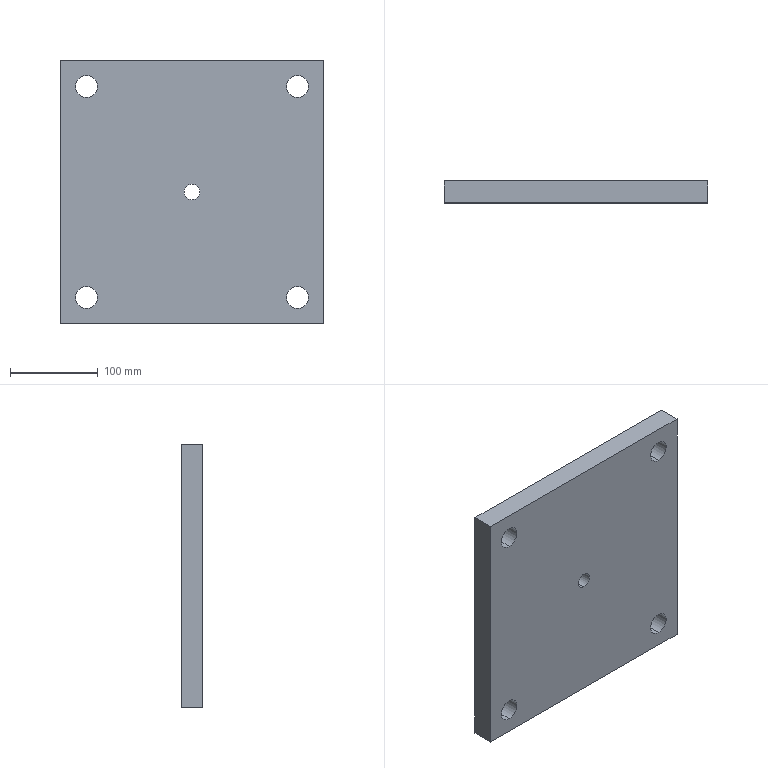Part | SolidWorks | features FlatPattern 1, SMBaseFlange 1, SheetMetal 1 | 1 solid | 16 faces | box 300 x 25 x 300 mm | volume 2194551 mm3 | cylinder 10 | plane 6 | commonest cylinder face diameters 25 x8 18 x2
STEP:
#1=CARTESIAN_POINT('',(-120.,-25.,-132.5));
#2=VERTEX_POINT('',#1);
#3=CARTESIAN_POINT('',(-120.,-25.,-107.5));
#4=VERTEX_POINT('',#3);
#5=CARTESIAN_POINT('',(-120.,-25.,-120.));
#6=DIRECTION('',(0.,1.,0.));
#7=DIRECTION('',(0.,0.,-1.));
#8=AXIS2_PLACEMENT_3D('',#5,#6,#7);
#9=CIRCLE('',#8,12.5);
#10=EDGE_CURVE('',#2,#4,#9,.T.);
#11=ORIENTED_EDGE('',*,*,#10,.F.);
#12=CARTESIAN_POINT('',(-120.,0.,-132.5));
#13=VERTEX_POINT('',#12);
#14=CARTESIAN_POINT('',(-120.,-25.,-132.5));
#15=DIRECTION('',(0.,1.,0.));
#16=VECTOR('',#15,1000.);
#17=LINE('',#14,#16);
#18=EDGE_CURVE('',#2,#13,#17,.T.);
#19=ORIENTED_EDGE('',*,*,#18,.T.);
#20=CARTESIAN_POINT('',(-120.,0.,-107.5));
#21=VERTEX_POINT('',#20);
#22=CARTESIAN_POINT('',(-120.,0.,-120.));
#23=DIRECTION('',(0.,1.,0.));
#24=DIRECTION('',(0.,0.,-1.));
#25=AXIS2_PLACEMENT_3D('',#22,#23,#24);
#26=CIRCLE('',#25,12.5);
#27=EDGE_CURVE('',#13,#21,#26,.T.);
#28=ORIENTED_EDGE('',*,*,#27,.T.);
#29=CARTESIAN_POINT('',(-120.,-25.,-107.5));
#30=DIRECTION('',(0.,1.,0.));
#31=VECTOR('',#30,1000.);
#32=LINE('',#29,#31);
#33=EDGE_CURVE('',#4,#21,#32,.T.);
#34=ORIENTED_EDGE('',*,*,#33,.F.);
#35=EDGE_LOOP('',(#11,#19,#28,#34));
#36=FACE_OUTER_BOUND('',#35,.T.);
#37=CARTESIAN_POINT('',(-120.,-25.,-120.));
#38=DIRECTION('',(0.,1.,0.));
#39=DIRECTION('',(0.,0.,1.));
#40=AXIS2_PLACEMENT_3D('',#37,#38,#39);
#41=CYLINDRICAL_SURFACE('',#40,12.5);
#42=ADVANCED_FACE('',(#36),#41,.F.);
#43=CARTESIAN_POINT('',(120.,-25.,-132.5));
#44=VERTEX_POINT('',#43);
#45=CARTESIAN_POINT('',(120.,-25.,-107.5));
#46=VERTEX_POINT('',#45);
#47=CARTESIAN_POINT('',(120.,-25.,-120.));
#48=DIRECTION('',(0.,1.,0.));
#49=DIRECTION('',(0.,0.,1.));
#50=AXIS2_PLACEMENT_3D('',#47,#48,#49);
#51=CIRCLE('',#50,12.5);
#52=EDGE_CURVE('',#44,#46,#51,.T.);
#53=ORIENTED_EDGE('',*,*,#52,.F.);
#54=CARTESIAN_POINT('',(120.,0.,-132.5));
#55=VERTEX_POINT('',#54);
#56=CARTESIAN_POINT('',(120.,-25.,-132.5));
#57=DIRECTION('',(0.,1.,0.));
#58=VECTOR('',#57,1000.);
#59=LINE('',#56,#58);
#60=EDGE_CURVE('',#44,#55,#59,.T.);
#61=ORIENTED_EDGE('',*,*,#60,.T.);
#62=CARTESIAN_POINT('',(120.,0.,-107.5));
#63=VERTEX_POINT('',#62);
#64=CARTESIAN_POINT('',(120.,0.,-120.));
#65=DIRECTION('',(0.,1.,0.));
#66=DIRECTION('',(0.,0.,1.));
#67=AXIS2_PLACEMENT_3D('',#64,#65,#66);
#68=CIRCLE('',#67,12.5);
#69=EDGE_CURVE('',#55,#63,#68,.T.);
#70=ORIENTED_EDGE('',*,*,#69,.T.);
#71=CARTESIAN_POINT('',(120.,-25.,-107.5));
#72=DIRECTION('',(0.,1.,0.));
#73=VECTOR('',#72,1000.);
#74=LINE('',#71,#73);
#75=EDGE_CURVE('',#46,#63,#74,.T.);
#76=ORIENTED_EDGE('',*,*,#75,.F.);
#77=EDGE_LOOP('',(#53,#61,#70,#76));
#78=FACE_OUTER_BOUND('',#77,.T.);
#79=CARTESIAN_POINT('',(120.,-25.,-120.));
#80=DIRECTION('',(0.,1.,0.));
#81=DIRECTION('',(0.,0.,1.));
#82=AXIS2_PLACEMENT_3D('',#79,#80,#81);
#83=CYLINDRICAL_SURFACE('',#82,12.5);
#84=ADVANCED_FACE('',(#78),#83,.F.);
#85=CARTESIAN_POINT('',(0.,-25.,-9.));
#86=VERTEX_POINT('',#85);
#87=CARTESIAN_POINT('',(0.,-25.,9.));
#88=VERTEX_POINT('',#87);
#89=CARTESIAN_POINT('',(0.,-25.,0.));
#90=DIRECTION('',(0.,1.,0.));
#91=DIRECTION('',(0.,0.,1.));
#92=AXIS2_PLACEMENT_3D('',#89,#90,#91);
#93=CIRCLE('',#92,9.);
#94=EDGE_CURVE('',#86,#88,#93,.T.);
#95=ORIENTED_EDGE('',*,*,#94,.F.);
#96=CARTESIAN_POINT('',(0.,0.,-9.));
#97=VERTEX_POINT('',#96);
#98=CARTESIAN_POINT('',(0.,-25.,-9.));
#99=DIRECTION('',(0.,1.,0.));
#100=VECTOR('',#99,1000.);
#101=LINE('',#98,#100);
#102=EDGE_CURVE('',#86,#97,#101,.T.);
#103=ORIENTED_EDGE('',*,*,#102,.T.);
#104=CARTESIAN_POINT('',(0.,0.,9.));
#105=VERTEX_POINT('',#104);
#106=CARTESIAN_POINT('',(0.,0.,0.));
#107=DIRECTION('',(0.,1.,0.));
#108=DIRECTION('',(0.,0.,1.));
#109=AXIS2_PLACEMENT_3D('',#106,#107,#108);
#110=CIRCLE('',#109,9.);
#111=EDGE_CURVE('',#97,#105,#110,.T.);
#112=ORIENTED_EDGE('',*,*,#111,.T.);
#113=CARTESIAN_POINT('',(0.,-25.,9.));
#114=DIRECTION('',(0.,1.,0.));
#115=VECTOR('',#114,1000.);
#116=LINE('',#113,#115);
#117=EDGE_CURVE('',#88,#105,#116,.T.);
#118=ORIENTED_EDGE('',*,*,#117,.F.);
#119=EDGE_LOOP('',(#95,#103,#112,#118));
#120=FACE_OUTER_BOUND('',#119,.T.);
#121=CARTESIAN_POINT('',(0.,-25.,0.));
#122=DIRECTION('',(0.,1.,0.));
#123=DIRECTION('',(0.,0.,1.));
#124=AXIS2_PLACEMENT_3D('',#121,#122,#123);
#125=CYLINDRICAL_SURFACE('',#124,9.);
#126=ADVANCED_FACE('',(#120),#125,.F.);
#127=CARTESIAN_POINT('',(120.,-25.,107.5));
#128=VERTEX_POINT('',#127);
#129=CARTESIAN_POINT('',(120.,-25.,132.5));
#130=VERTEX_POINT('',#129);
#131=CARTESIAN_POINT('',(120.,-25.,120.));
#132=DIRECTION('',(0.,1.,0.));
#133=DIRECTION('',(0.,0.,-1.));
#134=AXIS2_PLACEMENT_3D('',#131,#132,#133);
#135=CIRCLE('',#134,12.5);
#136=EDGE_CURVE('',#128,#130,#135,.T.);
#137=ORIENTED_EDGE('',*,*,#136,.F.);
#138=CARTESIAN_POINT('',(120.,0.,107.5));
#139=VERTEX_POINT('',#138);
#140=CARTESIAN_POINT('',(120.,-25.,107.5));
#141=DIRECTION('',(0.,1.,0.));
#142=VECTOR('',#141,1000.);
#143=LINE('',#140,#142);
#144=EDGE_CURVE('',#128,#139,#143,.T.);
#145=ORIENTED_EDGE('',*,*,#144,.T.);
#146=CARTESIAN_POINT('',(120.,0.,132.5));
#147=VERTEX_POINT('',#146);
#148=CARTESIAN_POINT('',(120.,0.,120.));
#149=DIRECTION('',(0.,1.,0.));
#150=DIRECTION('',(0.,0.,-1.));
#151=AXIS2_PLACEMENT_3D('',#148,#149,#150);
#152=CIRCLE('',#151,12.5);
#153=EDGE_CURVE('',#139,#147,#152,.T.);
#154=ORIENTED_EDGE('',*,*,#153,.T.);
#155=CARTESIAN_POINT('',(120.,-25.,132.5));
#156=DIRECTION('',(0.,1.,0.));
#157=VECTOR('',#156,1000.);
#158=LINE('',#155,#157);
#159=EDGE_CURVE('',#130,#147,#158,.T.);
#160=ORIENTED_EDGE('',*,*,#159,.F.);
#161=EDGE_LOOP('',(#137,#145,#154,#160));
#162=FACE_OUTER_BOUND('',#161,.T.);
#163=CARTESIAN_POINT('',(120.,-25.,120.));
#164=DIRECTION('',(0.,1.,0.));
#165=DIRECTION('',(0.,0.,1.));
#166=AXIS2_PLACEMENT_3D('',#163,#164,#165);
#167=CYLINDRICAL_SURFACE('',#166,12.5);
#168=ADVANCED_FACE('',(#162),#167,.F.);
#169=CARTESIAN_POINT('',(-120.,-25.,107.5));
#170=VERTEX_POINT('',#169);
#171=CARTESIAN_POINT('',(-120.,-25.,132.5));
#172=VERTEX_POINT('',#171);
#173=CARTESIAN_POINT('',(-120.,-25.,120.));
#174=DIRECTION('',(0.,1.,0.));
#175=DIRECTION('',(0.,0.,1.));
#176=AXIS2_PLACEMENT_3D('',#173,#174,#175);
#177=CIRCLE('',#176,12.5);
#178=EDGE_CURVE('',#170,#172,#177,.T.);
#179=ORIENTED_EDGE('',*,*,#178,.F.);
#180=CARTESIAN_POINT('',(-120.,0.,107.5));
#181=VERTEX_POINT('',#180);
#182=CARTESIAN_POINT('',(-120.,-25.,107.5));
#183=DIRECTION('',(0.,1.,0.));
#184=VECTOR('',#183,1000.);
#185=LINE('',#182,#184);
#186=EDGE_CURVE('',#170,#181,#185,.T.);
#187=ORIENTED_EDGE('',*,*,#186,.T.);
#188=CARTESIAN_POINT('',(-120.,0.,132.5));
#189=VERTEX_POINT('',#188);
#190=CARTESIAN_POINT('',(-120.,0.,120.));
#191=DIRECTION('',(0.,1.,0.));
#192=DIRECTION('',(0.,0.,1.));
#193=AXIS2_PLACEMENT_3D('',#190,#191,#192);
#194=CIRCLE('',#193,12.5);
#195=EDGE_CURVE('',#181,#189,#194,.T.);
#196=ORIENTED_EDGE('',*,*,#195,.T.);
#197=CARTESIAN_POINT('',(-120.,-25.,132.5));
#198=DIRECTION('',(0.,1.,0.));
#199=VECTOR('',#198,1000.);
#200=LINE('',#197,#199);
#201=EDGE_CURVE('',#172,#189,#200,.T.);
#202=ORIENTED_EDGE('',*,*,#201,.F.);
#203=EDGE_LOOP('',(#179,#187,#196,#202));
#204=FACE_OUTER_BOUND('',#203,.T.);
#205=CARTESIAN_POINT('',(-120.,-25.,120.));
#206=DIRECTION('',(0.,1.,0.));
#207=DIRECTION('',(0.,0.,1.));
#208=AXIS2_PLACEMENT_3D('',#205,#206,#207);
#209=CYLINDRICAL_SURFACE('',#208,12.5);
#210=ADVANCED_FACE('',(#204),#209,.F.);
#211=CARTESIAN_POINT('',(150.,0.,150.));
#212=VERTEX_POINT('',#211);
#213=CARTESIAN_POINT('',(150.,0.,-150.));
#214=VERTEX_POINT('',#213);
#215=CARTESIAN_POINT('',(150.,0.,-150.));
#216=DIRECTION('',(0.,0.,-1.));
#217=VECTOR('',#216,1000.);
#218=LINE('',#215,#217);
#219=EDGE_CURVE('',#212,#214,#218,.T.);
#220=ORIENTED_EDGE('',*,*,#219,.F.);
#221=CARTESIAN_POINT('',(150.,-25.,150.));
#222=VERTEX_POINT('',#221);
#223=CARTESIAN_POINT('',(150.,-25.,150.));
#224=DIRECTION('',(0.,1.,0.));
#225=VECTOR('',#224,1000.);
#226=LINE('',#223,#225);
#227=EDGE_CURVE('',#222,#212,#226,.T.);
#228=ORIENTED_EDGE('',*,*,#227,.F.);
#229=CARTESIAN_POINT('',(150.,-25.,-150.));
#230=VERTEX_POINT('',#229);
#231=CARTESIAN_POINT('',(150.,-25.,-150.));
#232=DIRECTION('',(0.,0.,-1.));
#233=VECTOR('',#232,1000.);
#234=LINE('',#231,#233);
#235=EDGE_CURVE('',#222,#230,#234,.T.);
#236=ORIENTED_EDGE('',*,*,#235,.T.);
#237=CARTESIAN_POINT('',(150.,-25.,-150.));
#238=DIRECTION('',(0.,1.,0.));
#239=VECTOR('',#238,1000.);
#240=LINE('',#237,#239);
#241=EDGE_CURVE('',#230,#214,#240,.T.);
#242=ORIENTED_EDGE('',*,*,#241,.T.);
#243=EDGE_LOOP('',(#220,#228,#236,#242));
#244=FACE_OUTER_BOUND('',#243,.T.);
#245=CARTESIAN_POINT('',(150.,-25.,-150.));
#246=DIRECTION('',(1.,0.,0.));
#247=DIRECTION('',(0.,0.,-1.));
#248=AXIS2_PLACEMENT_3D('',#245,#246,#247);
#249=PLANE('',#248);
#250=ADVANCED_FACE('',(#244),#249,.T.);
#251=CARTESIAN_POINT('',(-150.,0.,150.));
#252=VERTEX_POINT('',#251);
#253=CARTESIAN_POINT('',(-150.,0.,150.));
#254=DIRECTION('',(1.,0.,0.));
#255=VECTOR('',#254,1000.);
#256=LINE('',#253,#255);
#257=EDGE_CURVE('',#252,#212,#256,.T.);
#258=ORIENTED_EDGE('',*,*,#257,.F.);
#259=CARTESIAN_POINT('',(-150.,-25.,150.));
#260=VERTEX_POINT('',#259);
#261=CARTESIAN_POINT('',(-150.,-25.,150.));
#262=DIRECTION('',(0.,1.,0.));
#263=VECTOR('',#262,1000.);
#264=LINE('',#261,#263);
#265=EDGE_CURVE('',#260,#252,#264,.T.);
#266=ORIENTED_EDGE('',*,*,#265,.F.);
#267=CARTESIAN_POINT('',(-150.,-25.,150.));
#268=DIRECTION('',(1.,0.,0.));
#269=VECTOR('',#268,1000.);
#270=LINE('',#267,#269);
#271=EDGE_CURVE('',#260,#222,#270,.T.);
#272=ORIENTED_EDGE('',*,*,#271,.T.);
#273=ORIENTED_EDGE('',*,*,#227,.T.);
#274=EDGE_LOOP('',(#258,#266,#272,#273));
#275=FACE_OUTER_BOUND('',#274,.T.);
#276=CARTESIAN_POINT('',(-150.,-25.,150.));
#277=DIRECTION('',(0.,0.,1.));
#278=DIRECTION('',(1.,0.,0.));
#279=AXIS2_PLACEMENT_3D('',#276,#277,#278);
#280=PLANE('',#279);
#281=ADVANCED_FACE('',(#275),#280,.T.);
#282=CARTESIAN_POINT('',(-150.,0.,-150.));
#283=VERTEX_POINT('',#282);
#284=CARTESIAN_POINT('',(-150.,0.,-150.));
#285=DIRECTION('',(0.,0.,1.));
#286=VECTOR('',#285,1000.);
#287=LINE('',#284,#286);
#288=EDGE_CURVE('',#283,#252,#287,.T.);
#289=ORIENTED_EDGE('',*,*,#288,.F.);
#290=CARTESIAN_POINT('',(-150.,-25.,-150.));
#291=VERTEX_POINT('',#290);
#292=CARTESIAN_POINT('',(-150.,-25.,-150.));
#293=DIRECTION('',(0.,1.,0.));
#294=VECTOR('',#293,1000.);
#295=LINE('',#292,#294);
#296=EDGE_CURVE('',#291,#283,#295,.T.);
#297=ORIENTED_EDGE('',*,*,#296,.F.);
#298=CARTESIAN_POINT('',(-150.,-25.,-150.));
#299=DIRECTION('',(0.,0.,1.));
#300=VECTOR('',#299,1000.);
#301=LINE('',#298,#300);
#302=EDGE_CURVE('',#291,#260,#301,.T.);
#303=ORIENTED_EDGE('',*,*,#302,.T.);
#304=ORIENTED_EDGE('',*,*,#265,.T.);
#305=EDGE_LOOP('',(#289,#297,#303,#304));
#306=FACE_OUTER_BOUND('',#305,.T.);
#307=CARTESIAN_POINT('',(-150.,-25.,-150.));
#308=DIRECTION('',(-1.,0.,0.));
#309=DIRECTION('',(0.,0.,1.));
#310=AXIS2_PLACEMENT_3D('',#307,#308,#309);
#311=PLANE('',#310);
#312=ADVANCED_FACE('',(#306),#311,.T.);
#313=CARTESIAN_POINT('',(-150.,0.,-150.));
#314=DIRECTION('',(-1.,0.,0.));
#315=VECTOR('',#314,1000.);
#316=LINE('',#313,#315);
#317=EDGE_CURVE('',#214,#283,#316,.T.);
#318=ORIENTED_EDGE('',*,*,#317,.F.);
#319=ORIENTED_EDGE('',*,*,#241,.F.);
#320=CARTESIAN_POINT('',(-150.,-25.,-150.));
#321=DIRECTION('',(-1.,0.,0.));
#322=VECTOR('',#321,1000.);
#323=LINE('',#320,#322);
#324=EDGE_CURVE('',#230,#291,#323,.T.);
#325=ORIENTED_EDGE('',*,*,#324,.T.);
#326=ORIENTED_EDGE('',*,*,#296,.T.);
#327=EDGE_LOOP('',(#318,#319,#325,#326));
#328=FACE_OUTER_BOUND('',#327,.T.);
#329=CARTESIAN_POINT('',(-150.,-25.,-150.));
#330=DIRECTION('',(0.,0.,-1.));
#331=DIRECTION('',(-1.,0.,0.));
#332=AXIS2_PLACEMENT_3D('',#329,#330,#331);
#333=PLANE('',#332);
#334=ADVANCED_FACE('',(#328),#333,.T.);
#335=CARTESIAN_POINT('',(-120.,-25.,-120.));
#336=DIRECTION('',(0.,1.,0.));
#337=DIRECTION('',(0.,0.,-1.));
#338=AXIS2_PLACEMENT_3D('',#335,#336,#337);
#339=CIRCLE('',#338,12.5);
#340=EDGE_CURVE('',#4,#2,#339,.T.);
#341=ORIENTED_EDGE('',*,*,#340,.T.);
#342=ORIENTED_EDGE('',*,*,#10,.T.);
#343=EDGE_LOOP('',(#341,#342));
#344=FACE_BOUND('',#343,.T.);
#345=CARTESIAN_POINT('',(120.,-25.,-120.));
#346=DIRECTION('',(0.,1.,0.));
#347=DIRECTION('',(0.,0.,1.));
#348=AXIS2_PLACEMENT_3D('',#345,#346,#347);
#349=CIRCLE('',#348,12.5);
#350=EDGE_CURVE('',#46,#44,#349,.T.);
#351=ORIENTED_EDGE('',*,*,#350,.T.);
#352=ORIENTED_EDGE('',*,*,#52,.T.);
#353=EDGE_LOOP('',(#351,#352));
#354=FACE_BOUND('',#353,.T.);
#355=CARTESIAN_POINT('',(0.,-25.,0.));
#356=DIRECTION('',(0.,1.,0.));
#357=DIRECTION('',(0.,0.,1.));
#358=AXIS2_PLACEMENT_3D('',#355,#356,#357);
#359=CIRCLE('',#358,9.);
#360=EDGE_CURVE('',#88,#86,#359,.T.);
#361=ORIENTED_EDGE('',*,*,#360,.T.);
#362=ORIENTED_EDGE('',*,*,#94,.T.);
#363=EDGE_LOOP('',(#361,#362));
#364=FACE_BOUND('',#363,.T.);
#365=CARTESIAN_POINT('',(120.,-25.,120.));
#366=DIRECTION('',(0.,1.,0.));
#367=DIRECTION('',(0.,0.,-1.));
#368=AXIS2_PLACEMENT_3D('',#365,#366,#367);
#369=CIRCLE('',#368,12.5);
#370=EDGE_CURVE('',#130,#128,#369,.T.);
#371=ORIENTED_EDGE('',*,*,#370,.T.);
#372=ORIENTED_EDGE('',*,*,#136,.T.);
#373=EDGE_LOOP('',(#371,#372));
#374=FACE_BOUND('',#373,.T.);
#375=CARTESIAN_POINT('',(-120.,-25.,120.));
#376=DIRECTION('',(0.,1.,0.));
#377=DIRECTION('',(0.,0.,1.));
#378=AXIS2_PLACEMENT_3D('',#375,#376,#377);
#379=CIRCLE('',#378,12.5);
#380=EDGE_CURVE('',#172,#170,#379,.T.);
#381=ORIENTED_EDGE('',*,*,#380,.T.);
#382=ORIENTED_EDGE('',*,*,#178,.T.);
#383=EDGE_LOOP('',(#381,#382));
#384=FACE_BOUND('',#383,.T.);
#385=ORIENTED_EDGE('',*,*,#235,.F.);
#386=ORIENTED_EDGE('',*,*,#271,.F.);
#387=ORIENTED_EDGE('',*,*,#302,.F.);
#388=ORIENTED_EDGE('',*,*,#324,.F.);
#389=EDGE_LOOP('',(#385,#386,#387,#388));
#390=FACE_OUTER_BOUND('',#389,.T.);
#391=CARTESIAN_POINT('',(0.,-25.,0.));
#392=DIRECTION('',(0.,1.,0.));
#393=DIRECTION('',(0.,0.,1.));
#394=AXIS2_PLACEMENT_3D('',#391,#392,#393);
#395=PLANE('',#394);
#396=ADVANCED_FACE('',(#344,#354,#364,#374,#384,#390),#395,.F.);
#397=CARTESIAN_POINT('',(-120.,0.,-120.));
#398=DIRECTION('',(0.,1.,0.));
#399=DIRECTION('',(0.,0.,-1.));
#400=AXIS2_PLACEMENT_3D('',#397,#398,#399);
#401=CIRCLE('',#400,12.5);
#402=EDGE_CURVE('',#21,#13,#401,.T.);
#403=ORIENTED_EDGE('',*,*,#402,.F.);
#404=ORIENTED_EDGE('',*,*,#27,.F.);
#405=EDGE_LOOP('',(#403,#404));
#406=FACE_BOUND('',#405,.T.);
#407=CARTESIAN_POINT('',(120.,0.,-120.));
#408=DIRECTION('',(0.,1.,0.));
#409=DIRECTION('',(0.,0.,1.));
#410=AXIS2_PLACEMENT_3D('',#407,#408,#409);
#411=CIRCLE('',#410,12.5);
#412=EDGE_CURVE('',#63,#55,#411,.T.);
#413=ORIENTED_EDGE('',*,*,#412,.F.);
#414=ORIENTED_EDGE('',*,*,#69,.F.);
#415=EDGE_LOOP('',(#413,#414));
#416=FACE_BOUND('',#415,.T.);
#417=CARTESIAN_POINT('',(0.,0.,0.));
#418=DIRECTION('',(0.,1.,0.));
#419=DIRECTION('',(0.,0.,1.));
#420=AXIS2_PLACEMENT_3D('',#417,#418,#419);
#421=CIRCLE('',#420,9.);
#422=EDGE_CURVE('',#105,#97,#421,.T.);
#423=ORIENTED_EDGE('',*,*,#422,.F.);
#424=ORIENTED_EDGE('',*,*,#111,.F.);
#425=EDGE_LOOP('',(#423,#424));
#426=FACE_BOUND('',#425,.T.);
#427=CARTESIAN_POINT('',(120.,0.,120.));
#428=DIRECTION('',(0.,1.,0.));
#429=DIRECTION('',(0.,0.,-1.));
#430=AXIS2_PLACEMENT_3D('',#427,#428,#429);
#431=CIRCLE('',#430,12.5);
#432=EDGE_CURVE('',#147,#139,#431,.T.);
#433=ORIENTED_EDGE('',*,*,#432,.F.);
#434=ORIENTED_EDGE('',*,*,#153,.F.);
#435=EDGE_LOOP('',(#433,#434));
#436=FACE_BOUND('',#435,.T.);
#437=CARTESIAN_POINT('',(-120.,0.,120.));
#438=DIRECTION('',(0.,1.,0.));
#439=DIRECTION('',(0.,0.,1.));
#440=AXIS2_PLACEMENT_3D('',#437,#438,#439);
#441=CIRCLE('',#440,12.5);
#442=EDGE_CURVE('',#189,#181,#441,.T.);
#443=ORIENTED_EDGE('',*,*,#442,.F.);
#444=ORIENTED_EDGE('',*,*,#195,.F.);
#445=EDGE_LOOP('',(#443,#444));
#446=FACE_BOUND('',#445,.T.);
#447=ORIENTED_EDGE('',*,*,#219,.T.);
#448=ORIENTED_EDGE('',*,*,#317,.T.);
#449=ORIENTED_EDGE('',*,*,#288,.T.);
#450=ORIENTED_EDGE('',*,*,#257,.T.);
#451=EDGE_LOOP('',(#447,#448,#449,#450));
#452=FACE_OUTER_BOUND('',#451,.T.);
#453=CARTESIAN_POINT('',(0.,0.,0.));
#454=DIRECTION('',(0.,1.,0.));
#455=DIRECTION('',(0.,0.,1.));
#456=AXIS2_PLACEMENT_3D('',#453,#454,#455);
#457=PLANE('',#456);
#458=ADVANCED_FACE('',(#406,#416,#426,#436,#446,#452),#457,.T.);
#459=ORIENTED_EDGE('',*,*,#186,.F.);
#460=ORIENTED_EDGE('',*,*,#380,.F.);
#461=ORIENTED_EDGE('',*,*,#201,.T.);
#462=ORIENTED_EDGE('',*,*,#442,.T.);
#463=EDGE_LOOP('',(#459,#460,#461,#462));
#464=FACE_OUTER_BOUND('',#463,.T.);
#465=CARTESIAN_POINT('',(-120.,-25.,120.));
#466=DIRECTION('',(0.,1.,0.));
#467=DIRECTION('',(0.,0.,1.));
#468=AXIS2_PLACEMENT_3D('',#465,#466,#467);
#469=CYLINDRICAL_SURFACE('',#468,12.5);
#470=ADVANCED_FACE('',(#464),#469,.F.);
#471=ORIENTED_EDGE('',*,*,#144,.F.);
#472=ORIENTED_EDGE('',*,*,#370,.F.);
#473=ORIENTED_EDGE('',*,*,#159,.T.);
#474=ORIENTED_EDGE('',*,*,#432,.T.);
#475=EDGE_LOOP('',(#471,#472,#473,#474));
#476=FACE_OUTER_BOUND('',#475,.T.);
#477=CARTESIAN_POINT('',(120.,-25.,120.));
#478=DIRECTION('',(0.,1.,0.));
#479=DIRECTION('',(0.,0.,1.));
#480=AXIS2_PLACEMENT_3D('',#477,#478,#479);
#481=CYLINDRICAL_SURFACE('',#480,12.5);
#482=ADVANCED_FACE('',(#476),#481,.F.);
#483=ORIENTED_EDGE('',*,*,#102,.F.);
#484=ORIENTED_EDGE('',*,*,#360,.F.);
#485=ORIENTED_EDGE('',*,*,#117,.T.);
#486=ORIENTED_EDGE('',*,*,#422,.T.);
#487=EDGE_LOOP('',(#483,#484,#485,#486));
#488=FACE_OUTER_BOUND('',#487,.T.);
#489=CARTESIAN_POINT('',(0.,-25.,0.));
#490=DIRECTION('',(0.,1.,0.));
#491=DIRECTION('',(0.,0.,1.));
#492=AXIS2_PLACEMENT_3D('',#489,#490,#491);
#493=CYLINDRICAL_SURFACE('',#492,9.);
#494=ADVANCED_FACE('',(#488),#493,.F.);
#495=ORIENTED_EDGE('',*,*,#60,.F.);
#496=ORIENTED_EDGE('',*,*,#350,.F.);
#497=ORIENTED_EDGE('',*,*,#75,.T.);
#498=ORIENTED_EDGE('',*,*,#412,.T.);
#499=EDGE_LOOP('',(#495,#496,#497,#498));
#500=FACE_OUTER_BOUND('',#499,.T.);
#501=CARTESIAN_POINT('',(120.,-25.,-120.));
#502=DIRECTION('',(0.,1.,0.));
#503=DIRECTION('',(0.,0.,1.));
#504=AXIS2_PLACEMENT_3D('',#501,#502,#503);
#505=CYLINDRICAL_SURFACE('',#504,12.5);
#506=ADVANCED_FACE('',(#500),#505,.F.);
#507=ORIENTED_EDGE('',*,*,#18,.F.);
#508=ORIENTED_EDGE('',*,*,#340,.F.);
#509=ORIENTED_EDGE('',*,*,#33,.T.);
#510=ORIENTED_EDGE('',*,*,#402,.T.);
#511=EDGE_LOOP('',(#507,#508,#509,#510));
#512=FACE_OUTER_BOUND('',#511,.T.);
#513=CARTESIAN_POINT('',(-120.,-25.,-120.));
#514=DIRECTION('',(0.,1.,0.));
#515=DIRECTION('',(0.,0.,1.));
#516=AXIS2_PLACEMENT_3D('',#513,#514,#515);
#517=CYLINDRICAL_SURFACE('',#516,12.5);
#518=ADVANCED_FACE('',(#512),#517,.F.);
#519=CLOSED_SHELL('',(#42,#84,#126,#168,#210,#250,#281,#312,#334,#396,#458,#470,#482,#494,#506,#518));
#520=MANIFOLD_SOLID_BREP('',#519);
#521=CARTESIAN_POINT('',(0.,0.,0.));
#522=DIRECTION('',(0.,0.,1.));
#523=DIRECTION('',(1.,0.,0.));
#524=AXIS2_PLACEMENT_3D('',#521,#522,#523);
#525=(LENGTH_UNIT()NAMED_UNIT(*)SI_UNIT(.MILLI.,.METRE.));
#526=UNCERTAINTY_MEASURE_WITH_UNIT(LENGTH_MEASURE(0.00001),#525,'','');
#527=(NAMED_UNIT(*)PLANE_ANGLE_UNIT()SI_UNIT($,.RADIAN.));
#528=(NAMED_UNIT(*)SI_UNIT($,.STERADIAN.)SOLID_ANGLE_UNIT());
#529=(GEOMETRIC_REPRESENTATION_CONTEXT(3)GLOBAL_UNCERTAINTY_ASSIGNED_CONTEXT((#526))GLOBAL_UNIT_ASSIGNED_CONTEXT((#525,#527,#528))REPRESENTATION_CONTEXT('',''));
#530=ADVANCED_BREP_SHAPE_REPRESENTATION('',(#520,#524),#529);